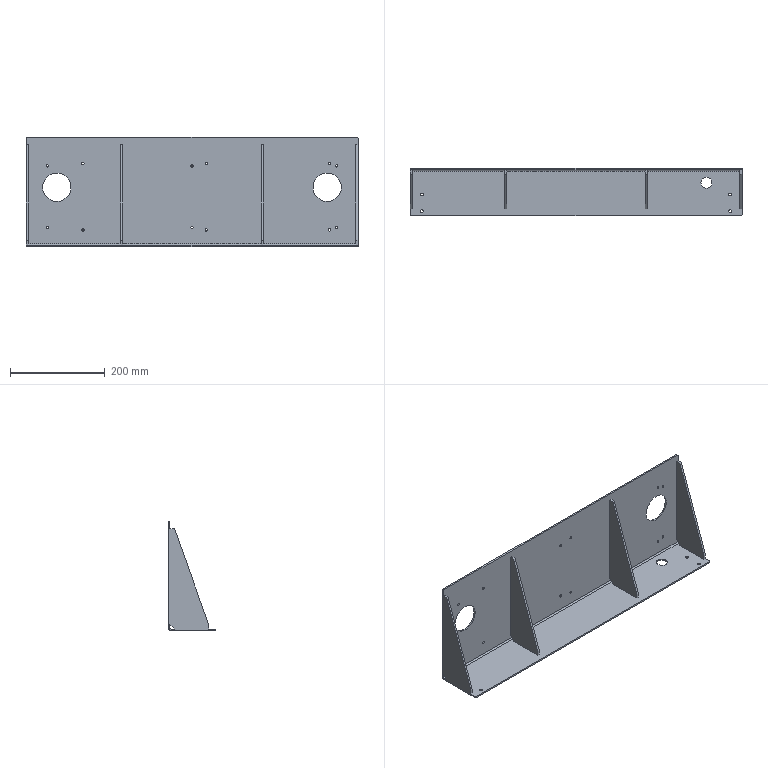Part | STEP file | 227H056114 BKT Default | 3 solids | 82 faces | box 700 x 100 x 230 mm | volume 887594 mm3 | plane 42 | cylinder 40 | commonest cylinder face diameters 5 x24 6 x9 60 x4 23 x2 12.4 x1